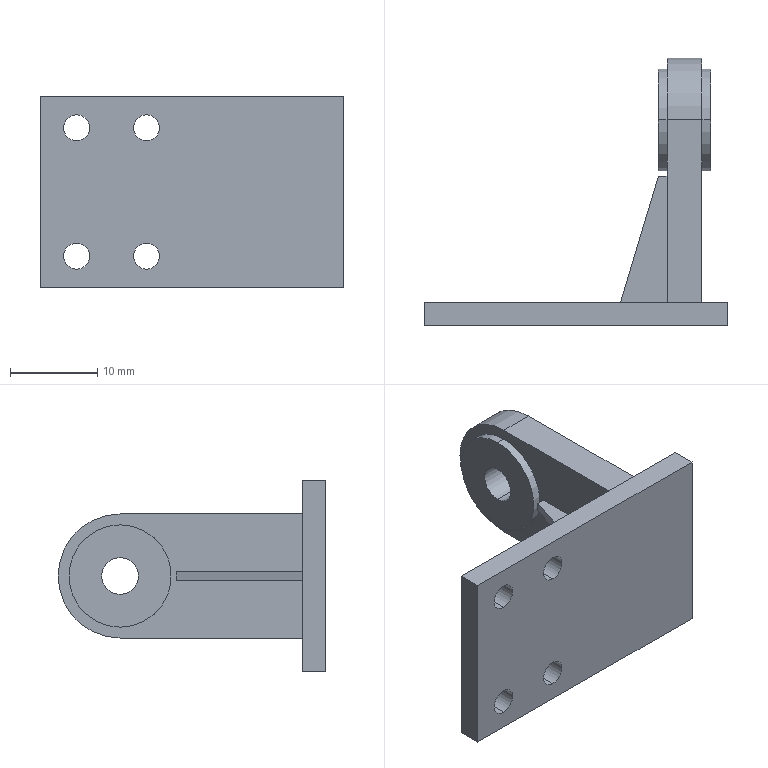Part | SolidWorks | features SavedExtBody 1 | 1 solid | 31 faces | box 34.775 x 30.759 x 22 mm | volume 3678 mm3 | plane 16 | cylinder 15 | commonest cylinder face diameters 3 x8 11.749 x4 4.217 x2 14.248 x1
STEP:
#1=CARTESIAN_POINT('',(69.335,-225.404,73.872));
#2=VERTEX_POINT('',#1);
#3=CARTESIAN_POINT('',(69.335,-225.404,70.872));
#4=VERTEX_POINT('',#3);
#5=CARTESIAN_POINT('',(69.335,-225.404,72.372));
#6=DIRECTION('',(0.,-1.,0.));
#7=DIRECTION('',(0.,0.,-1.));
#8=AXIS2_PLACEMENT_3D('',#5,#6,#7);
#9=CIRCLE('',#8,1.5);
#10=EDGE_CURVE('',#2,#4,#9,.T.);
#11=ORIENTED_EDGE('',*,*,#10,.F.);
#12=CARTESIAN_POINT('',(69.335,-228.101,73.872));
#13=VERTEX_POINT('',#12);
#14=CARTESIAN_POINT('',(69.335,-217.763,73.872));
#15=DIRECTION('',(0.,-1.,0.));
#16=VECTOR('',#15,1000.);
#17=LINE('',#14,#16);
#18=EDGE_CURVE('',#2,#13,#17,.T.);
#19=ORIENTED_EDGE('',*,*,#18,.T.);
#20=CARTESIAN_POINT('',(69.335,-228.101,70.872));
#21=VERTEX_POINT('',#20);
#22=CARTESIAN_POINT('',(69.335,-228.101,72.372));
#23=DIRECTION('',(0.,1.,0.));
#24=DIRECTION('',(0.,0.,1.));
#25=AXIS2_PLACEMENT_3D('',#22,#23,#24);
#26=CIRCLE('',#25,1.5);
#27=EDGE_CURVE('',#21,#13,#26,.T.);
#28=ORIENTED_EDGE('',*,*,#27,.F.);
#29=CARTESIAN_POINT('',(69.335,-217.763,70.872));
#30=DIRECTION('',(0.,-1.,0.));
#31=VECTOR('',#30,1000.);
#32=LINE('',#29,#31);
#33=EDGE_CURVE('',#4,#21,#32,.T.);
#34=ORIENTED_EDGE('',*,*,#33,.F.);
#35=EDGE_LOOP('',(#11,#19,#28,#34));
#36=FACE_OUTER_BOUND('',#35,.T.);
#37=CARTESIAN_POINT('',(69.335,-217.763,72.372));
#38=DIRECTION('',(0.,-1.,0.));
#39=DIRECTION('',(0.,0.,-1.));
#40=AXIS2_PLACEMENT_3D('',#37,#38,#39);
#41=CYLINDRICAL_SURFACE('',#40,1.5);
#42=ADVANCED_FACE('',(#36),#41,.F.);
#43=CARTESIAN_POINT('',(77.361,-225.404,73.872));
#44=VERTEX_POINT('',#43);
#45=CARTESIAN_POINT('',(77.361,-225.404,70.872));
#46=VERTEX_POINT('',#45);
#47=CARTESIAN_POINT('',(77.361,-225.404,72.372));
#48=DIRECTION('',(0.,-1.,0.));
#49=DIRECTION('',(0.,0.,-1.));
#50=AXIS2_PLACEMENT_3D('',#47,#48,#49);
#51=CIRCLE('',#50,1.5);
#52=EDGE_CURVE('',#44,#46,#51,.T.);
#53=ORIENTED_EDGE('',*,*,#52,.F.);
#54=CARTESIAN_POINT('',(77.361,-228.101,73.872));
#55=VERTEX_POINT('',#54);
#56=CARTESIAN_POINT('',(77.361,-217.763,73.872));
#57=DIRECTION('',(0.,-1.,0.));
#58=VECTOR('',#57,1000.);
#59=LINE('',#56,#58);
#60=EDGE_CURVE('',#44,#55,#59,.T.);
#61=ORIENTED_EDGE('',*,*,#60,.T.);
#62=CARTESIAN_POINT('',(77.361,-228.101,70.872));
#63=VERTEX_POINT('',#62);
#64=CARTESIAN_POINT('',(77.361,-228.101,72.372));
#65=DIRECTION('',(0.,1.,0.));
#66=DIRECTION('',(0.,0.,1.));
#67=AXIS2_PLACEMENT_3D('',#64,#65,#66);
#68=CIRCLE('',#67,1.5);
#69=EDGE_CURVE('',#63,#55,#68,.T.);
#70=ORIENTED_EDGE('',*,*,#69,.F.);
#71=CARTESIAN_POINT('',(77.361,-217.763,70.872));
#72=DIRECTION('',(0.,-1.,0.));
#73=VECTOR('',#72,1000.);
#74=LINE('',#71,#73);
#75=EDGE_CURVE('',#46,#63,#74,.T.);
#76=ORIENTED_EDGE('',*,*,#75,.F.);
#77=EDGE_LOOP('',(#53,#61,#70,#76));
#78=FACE_OUTER_BOUND('',#77,.T.);
#79=CARTESIAN_POINT('',(77.361,-217.763,72.372));
#80=DIRECTION('',(0.,-1.,0.));
#81=DIRECTION('',(0.,0.,-1.));
#82=AXIS2_PLACEMENT_3D('',#79,#80,#81);
#83=CYLINDRICAL_SURFACE('',#82,1.5);
#84=ADVANCED_FACE('',(#78),#83,.F.);
#85=CARTESIAN_POINT('',(77.361,-225.404,59.128));
#86=VERTEX_POINT('',#85);
#87=CARTESIAN_POINT('',(77.361,-225.404,56.128));
#88=VERTEX_POINT('',#87);
#89=CARTESIAN_POINT('',(77.361,-225.404,57.628));
#90=DIRECTION('',(0.,-1.,0.));
#91=DIRECTION('',(0.,0.,-1.));
#92=AXIS2_PLACEMENT_3D('',#89,#90,#91);
#93=CIRCLE('',#92,1.5);
#94=EDGE_CURVE('',#86,#88,#93,.T.);
#95=ORIENTED_EDGE('',*,*,#94,.F.);
#96=CARTESIAN_POINT('',(77.361,-228.101,59.128));
#97=VERTEX_POINT('',#96);
#98=CARTESIAN_POINT('',(77.361,-217.763,59.128));
#99=DIRECTION('',(0.,-1.,0.));
#100=VECTOR('',#99,1000.);
#101=LINE('',#98,#100);
#102=EDGE_CURVE('',#86,#97,#101,.T.);
#103=ORIENTED_EDGE('',*,*,#102,.T.);
#104=CARTESIAN_POINT('',(77.361,-228.101,56.128));
#105=VERTEX_POINT('',#104);
#106=CARTESIAN_POINT('',(77.361,-228.101,57.628));
#107=DIRECTION('',(0.,1.,0.));
#108=DIRECTION('',(0.,0.,1.));
#109=AXIS2_PLACEMENT_3D('',#106,#107,#108);
#110=CIRCLE('',#109,1.5);
#111=EDGE_CURVE('',#105,#97,#110,.T.);
#112=ORIENTED_EDGE('',*,*,#111,.F.);
#113=CARTESIAN_POINT('',(77.361,-217.763,56.128));
#114=DIRECTION('',(0.,-1.,0.));
#115=VECTOR('',#114,1000.);
#116=LINE('',#113,#115);
#117=EDGE_CURVE('',#88,#105,#116,.T.);
#118=ORIENTED_EDGE('',*,*,#117,.F.);
#119=EDGE_LOOP('',(#95,#103,#112,#118));
#120=FACE_OUTER_BOUND('',#119,.T.);
#121=CARTESIAN_POINT('',(77.361,-217.763,57.628));
#122=DIRECTION('',(0.,-1.,0.));
#123=DIRECTION('',(0.,0.,-1.));
#124=AXIS2_PLACEMENT_3D('',#121,#122,#123);
#125=CYLINDRICAL_SURFACE('',#124,1.5);
#126=ADVANCED_FACE('',(#120),#125,.F.);
#127=CARTESIAN_POINT('',(69.335,-225.404,59.128));
#128=VERTEX_POINT('',#127);
#129=CARTESIAN_POINT('',(69.335,-225.404,56.128));
#130=VERTEX_POINT('',#129);
#131=CARTESIAN_POINT('',(69.335,-225.404,57.628));
#132=DIRECTION('',(0.,-1.,0.));
#133=DIRECTION('',(0.,0.,-1.));
#134=AXIS2_PLACEMENT_3D('',#131,#132,#133);
#135=CIRCLE('',#134,1.5);
#136=EDGE_CURVE('',#128,#130,#135,.T.);
#137=ORIENTED_EDGE('',*,*,#136,.F.);
#138=CARTESIAN_POINT('',(69.335,-228.101,59.128));
#139=VERTEX_POINT('',#138);
#140=CARTESIAN_POINT('',(69.335,-217.763,59.128));
#141=DIRECTION('',(0.,-1.,0.));
#142=VECTOR('',#141,1000.);
#143=LINE('',#140,#142);
#144=EDGE_CURVE('',#128,#139,#143,.T.);
#145=ORIENTED_EDGE('',*,*,#144,.T.);
#146=CARTESIAN_POINT('',(69.335,-228.101,56.128));
#147=VERTEX_POINT('',#146);
#148=CARTESIAN_POINT('',(69.335,-228.101,57.628));
#149=DIRECTION('',(0.,1.,0.));
#150=DIRECTION('',(0.,0.,1.));
#151=AXIS2_PLACEMENT_3D('',#148,#149,#150);
#152=CIRCLE('',#151,1.5);
#153=EDGE_CURVE('',#147,#139,#152,.T.);
#154=ORIENTED_EDGE('',*,*,#153,.F.);
#155=CARTESIAN_POINT('',(69.335,-217.763,56.128));
#156=DIRECTION('',(0.,-1.,0.));
#157=VECTOR('',#156,1000.);
#158=LINE('',#155,#157);
#159=EDGE_CURVE('',#130,#147,#158,.T.);
#160=ORIENTED_EDGE('',*,*,#159,.F.);
#161=EDGE_LOOP('',(#137,#145,#154,#160));
#162=FACE_OUTER_BOUND('',#161,.T.);
#163=CARTESIAN_POINT('',(69.335,-217.763,57.628));
#164=DIRECTION('',(0.,-1.,0.));
#165=DIRECTION('',(0.,0.,-1.));
#166=AXIS2_PLACEMENT_3D('',#163,#164,#165);
#167=CYLINDRICAL_SURFACE('',#166,1.5);
#168=ADVANCED_FACE('',(#162),#167,.F.);
#169=CARTESIAN_POINT('',(92.041,-204.466,67.108));
#170=VERTEX_POINT('',#169);
#171=CARTESIAN_POINT('',(92.041,-204.466,62.892));
#172=VERTEX_POINT('',#171);
#173=CARTESIAN_POINT('',(92.041,-204.466,65.));
#174=DIRECTION('',(1.,0.,0.));
#175=DIRECTION('',(0.,0.,-1.));
#176=AXIS2_PLACEMENT_3D('',#173,#174,#175);
#177=CIRCLE('',#176,2.108);
#178=EDGE_CURVE('',#170,#172,#177,.T.);
#179=ORIENTED_EDGE('',*,*,#178,.F.);
#180=CARTESIAN_POINT('',(98.041,-204.466,67.108));
#181=VERTEX_POINT('',#180);
#182=CARTESIAN_POINT('',(100.386,-204.466,67.108));
#183=DIRECTION('',(1.,0.,0.));
#184=VECTOR('',#183,1000.);
#185=LINE('',#182,#184);
#186=EDGE_CURVE('',#170,#181,#185,.T.);
#187=ORIENTED_EDGE('',*,*,#186,.T.);
#188=CARTESIAN_POINT('',(98.041,-204.466,62.892));
#189=VERTEX_POINT('',#188);
#190=CARTESIAN_POINT('',(98.041,-204.466,65.));
#191=DIRECTION('',(1.,0.,0.));
#192=DIRECTION('',(0.,0.,-1.));
#193=AXIS2_PLACEMENT_3D('',#190,#191,#192);
#194=CIRCLE('',#193,2.108);
#195=EDGE_CURVE('',#181,#189,#194,.T.);
#196=ORIENTED_EDGE('',*,*,#195,.T.);
#197=CARTESIAN_POINT('',(100.386,-204.466,62.892));
#198=DIRECTION('',(1.,0.,0.));
#199=VECTOR('',#198,1000.);
#200=LINE('',#197,#199);
#201=EDGE_CURVE('',#172,#189,#200,.T.);
#202=ORIENTED_EDGE('',*,*,#201,.F.);
#203=EDGE_LOOP('',(#179,#187,#196,#202));
#204=FACE_OUTER_BOUND('',#203,.T.);
#205=CARTESIAN_POINT('',(100.386,-204.466,65.));
#206=DIRECTION('',(1.,0.,0.));
#207=DIRECTION('',(0.,0.,-1.));
#208=AXIS2_PLACEMENT_3D('',#205,#206,#207);
#209=CYLINDRICAL_SURFACE('',#208,2.108);
#210=ADVANCED_FACE('',(#204),#209,.F.);
#211=CARTESIAN_POINT('',(98.041,-204.466,59.125));
#212=VERTEX_POINT('',#211);
#213=CARTESIAN_POINT('',(98.041,-204.466,70.875));
#214=VERTEX_POINT('',#213);
#215=CARTESIAN_POINT('',(98.041,-204.466,65.));
#216=DIRECTION('',(1.,0.,0.));
#217=DIRECTION('',(0.,0.,-1.));
#218=AXIS2_PLACEMENT_3D('',#215,#216,#217);
#219=CIRCLE('',#218,5.875);
#220=EDGE_CURVE('',#212,#214,#219,.T.);
#221=ORIENTED_EDGE('',*,*,#220,.F.);
#222=CARTESIAN_POINT('',(97.041,-204.466,59.125));
#223=VERTEX_POINT('',#222);
#224=CARTESIAN_POINT('',(98.041,-204.466,59.125));
#225=DIRECTION('',(-1.,0.,0.));
#226=VECTOR('',#225,1000.);
#227=LINE('',#224,#226);
#228=EDGE_CURVE('',#212,#223,#227,.T.);
#229=ORIENTED_EDGE('',*,*,#228,.T.);
#230=CARTESIAN_POINT('',(97.041,-204.466,70.875));
#231=VERTEX_POINT('',#230);
#232=CARTESIAN_POINT('',(97.041,-204.466,65.));
#233=DIRECTION('',(-1.,0.,0.));
#234=DIRECTION('',(0.,0.,-1.));
#235=AXIS2_PLACEMENT_3D('',#232,#233,#234);
#236=CIRCLE('',#235,5.875);
#237=EDGE_CURVE('',#231,#223,#236,.T.);
#238=ORIENTED_EDGE('',*,*,#237,.F.);
#239=CARTESIAN_POINT('',(98.041,-204.466,70.875));
#240=DIRECTION('',(-1.,0.,0.));
#241=VECTOR('',#240,1000.);
#242=LINE('',#239,#241);
#243=EDGE_CURVE('',#214,#231,#242,.T.);
#244=ORIENTED_EDGE('',*,*,#243,.F.);
#245=EDGE_LOOP('',(#221,#229,#238,#244));
#246=FACE_OUTER_BOUND('',#245,.T.);
#247=CARTESIAN_POINT('',(98.041,-204.466,65.));
#248=DIRECTION('',(-1.,0.,0.));
#249=DIRECTION('',(0.,0.,1.));
#250=AXIS2_PLACEMENT_3D('',#247,#248,#249);
#251=CYLINDRICAL_SURFACE('',#250,5.875);
#252=ADVANCED_FACE('',(#246),#251,.T.);
#253=CARTESIAN_POINT('',(93.041,-204.466,70.875));
#254=VERTEX_POINT('',#253);
#255=CARTESIAN_POINT('',(93.041,-204.466,59.125));
#256=VERTEX_POINT('',#255);
#257=CARTESIAN_POINT('',(93.041,-204.466,65.));
#258=DIRECTION('',(-1.,0.,0.));
#259=DIRECTION('',(0.,0.,-1.));
#260=AXIS2_PLACEMENT_3D('',#257,#258,#259);
#261=CIRCLE('',#260,5.875);
#262=EDGE_CURVE('',#254,#256,#261,.T.);
#263=ORIENTED_EDGE('',*,*,#262,.T.);
#264=CARTESIAN_POINT('',(92.041,-204.466,59.125));
#265=VERTEX_POINT('',#264);
#266=CARTESIAN_POINT('',(98.041,-204.466,59.125));
#267=DIRECTION('',(-1.,0.,0.));
#268=VECTOR('',#267,1000.);
#269=LINE('',#266,#268);
#270=EDGE_CURVE('',#256,#265,#269,.T.);
#271=ORIENTED_EDGE('',*,*,#270,.T.);
#272=CARTESIAN_POINT('',(92.041,-204.466,70.875));
#273=VERTEX_POINT('',#272);
#274=CARTESIAN_POINT('',(92.041,-204.466,65.));
#275=DIRECTION('',(1.,0.,0.));
#276=DIRECTION('',(0.,0.,-1.));
#277=AXIS2_PLACEMENT_3D('',#274,#275,#276);
#278=CIRCLE('',#277,5.875);
#279=EDGE_CURVE('',#265,#273,#278,.T.);
#280=ORIENTED_EDGE('',*,*,#279,.T.);
#281=CARTESIAN_POINT('',(98.041,-204.466,70.875));
#282=DIRECTION('',(-1.,0.,0.));
#283=VECTOR('',#282,1000.);
#284=LINE('',#281,#283);
#285=EDGE_CURVE('',#254,#273,#284,.T.);
#286=ORIENTED_EDGE('',*,*,#285,.F.);
#287=EDGE_LOOP('',(#263,#271,#280,#286));
#288=FACE_OUTER_BOUND('',#287,.T.);
#289=CARTESIAN_POINT('',(98.041,-204.466,65.));
#290=DIRECTION('',(-1.,0.,0.));
#291=DIRECTION('',(0.,0.,1.));
#292=AXIS2_PLACEMENT_3D('',#289,#290,#291);
#293=CYLINDRICAL_SURFACE('',#292,5.875);
#294=ADVANCED_FACE('',(#288),#293,.T.);
#295=CARTESIAN_POINT('',(65.198,-225.404,54.));
#296=VERTEX_POINT('',#295);
#297=CARTESIAN_POINT('',(65.198,-228.101,54.));
#298=VERTEX_POINT('',#297);
#299=CARTESIAN_POINT('',(65.198,-228.101,54.));
#300=DIRECTION('',(0.,-1.,0.));
#301=VECTOR('',#300,1000.);
#302=LINE('',#299,#301);
#303=EDGE_CURVE('',#296,#298,#302,.T.);
#304=ORIENTED_EDGE('',*,*,#303,.T.);
#305=CARTESIAN_POINT('',(65.198,-228.101,76.));
#306=VERTEX_POINT('',#305);
#307=CARTESIAN_POINT('',(65.198,-228.101,76.));
#308=DIRECTION('',(0.,0.,-1.));
#309=VECTOR('',#308,1000.);
#310=LINE('',#307,#309);
#311=EDGE_CURVE('',#306,#298,#310,.T.);
#312=ORIENTED_EDGE('',*,*,#311,.F.);
#313=CARTESIAN_POINT('',(65.198,-225.404,76.));
#314=VERTEX_POINT('',#313);
#315=CARTESIAN_POINT('',(65.198,-228.101,76.));
#316=DIRECTION('',(0.,-1.,0.));
#317=VECTOR('',#316,1000.);
#318=LINE('',#315,#317);
#319=EDGE_CURVE('',#314,#306,#318,.T.);
#320=ORIENTED_EDGE('',*,*,#319,.F.);
#321=CARTESIAN_POINT('',(65.198,-225.404,76.));
#322=DIRECTION('',(0.,0.,-1.));
#323=VECTOR('',#322,1000.);
#324=LINE('',#321,#323);
#325=EDGE_CURVE('',#314,#296,#324,.T.);
#326=ORIENTED_EDGE('',*,*,#325,.T.);
#327=EDGE_LOOP('',(#304,#312,#320,#326));
#328=FACE_OUTER_BOUND('',#327,.T.);
#329=CARTESIAN_POINT('',(65.198,-228.101,76.));
#330=DIRECTION('',(1.,0.,0.));
#331=DIRECTION('',(0.,0.,-1.));
#332=AXIS2_PLACEMENT_3D('',#329,#330,#331);
#333=PLANE('',#332);
#334=ADVANCED_FACE('',(#328),#333,.F.);
#335=ORIENTED_EDGE('',*,*,#27,.T.);
#336=CARTESIAN_POINT('',(69.335,-228.101,72.372));
#337=DIRECTION('',(0.,1.,0.));
#338=DIRECTION('',(0.,0.,1.));
#339=AXIS2_PLACEMENT_3D('',#336,#337,#338);
#340=CIRCLE('',#339,1.5);
#341=EDGE_CURVE('',#13,#21,#340,.T.);
#342=ORIENTED_EDGE('',*,*,#341,.T.);
#343=EDGE_LOOP('',(#335,#342));
#344=FACE_BOUND('',#343,.T.);
#345=ORIENTED_EDGE('',*,*,#69,.T.);
#346=CARTESIAN_POINT('',(77.361,-228.101,72.372));
#347=DIRECTION('',(0.,1.,0.));
#348=DIRECTION('',(0.,0.,1.));
#349=AXIS2_PLACEMENT_3D('',#346,#347,#348);
#350=CIRCLE('',#349,1.5);
#351=EDGE_CURVE('',#55,#63,#350,.T.);
#352=ORIENTED_EDGE('',*,*,#351,.T.);
#353=EDGE_LOOP('',(#345,#352));
#354=FACE_BOUND('',#353,.T.);
#355=ORIENTED_EDGE('',*,*,#111,.T.);
#356=CARTESIAN_POINT('',(77.361,-228.101,57.628));
#357=DIRECTION('',(0.,1.,0.));
#358=DIRECTION('',(0.,0.,1.));
#359=AXIS2_PLACEMENT_3D('',#356,#357,#358);
#360=CIRCLE('',#359,1.5);
#361=EDGE_CURVE('',#97,#105,#360,.T.);
#362=ORIENTED_EDGE('',*,*,#361,.T.);
#363=EDGE_LOOP('',(#355,#362));
#364=FACE_BOUND('',#363,.T.);
#365=ORIENTED_EDGE('',*,*,#153,.T.);
#366=CARTESIAN_POINT('',(69.335,-228.101,57.628));
#367=DIRECTION('',(0.,1.,0.));
#368=DIRECTION('',(0.,0.,1.));
#369=AXIS2_PLACEMENT_3D('',#366,#367,#368);
#370=CIRCLE('',#369,1.5);
#371=EDGE_CURVE('',#139,#147,#370,.T.);
#372=ORIENTED_EDGE('',*,*,#371,.T.);
#373=EDGE_LOOP('',(#365,#372));
#374=FACE_BOUND('',#373,.T.);
#375=CARTESIAN_POINT('',(99.974,-228.101,54.));
#376=VERTEX_POINT('',#375);
#377=CARTESIAN_POINT('',(65.198,-228.101,54.));
#378=DIRECTION('',(1.,0.,0.));
#379=VECTOR('',#378,1000.);
#380=LINE('',#377,#379);
#381=EDGE_CURVE('',#298,#376,#380,.T.);
#382=ORIENTED_EDGE('',*,*,#381,.T.);
#383=CARTESIAN_POINT('',(99.974,-228.101,76.));
#384=VERTEX_POINT('',#383);
#385=CARTESIAN_POINT('',(99.974,-228.101,76.));
#386=DIRECTION('',(0.,0.,-1.));
#387=VECTOR('',#386,1000.);
#388=LINE('',#385,#387);
#389=EDGE_CURVE('',#384,#376,#388,.T.);
#390=ORIENTED_EDGE('',*,*,#389,.F.);
#391=CARTESIAN_POINT('',(65.198,-228.101,76.));
#392=DIRECTION('',(1.,0.,0.));
#393=VECTOR('',#392,1000.);
#394=LINE('',#391,#393);
#395=EDGE_CURVE('',#306,#384,#394,.T.);
#396=ORIENTED_EDGE('',*,*,#395,.F.);
#397=ORIENTED_EDGE('',*,*,#311,.T.);
#398=EDGE_LOOP('',(#382,#390,#396,#397));
#399=FACE_OUTER_BOUND('',#398,.T.);
#400=CARTESIAN_POINT('',(65.198,-228.101,76.));
#401=DIRECTION('',(0.,1.,0.));
#402=DIRECTION('',(0.,0.,1.));
#403=AXIS2_PLACEMENT_3D('',#400,#401,#402);
#404=PLANE('',#403);
#405=ADVANCED_FACE('',(#344,#354,#364,#374,#399),#404,.F.);
#406=CARTESIAN_POINT('',(99.974,-225.404,54.));
#407=VERTEX_POINT('',#406);
#408=CARTESIAN_POINT('',(99.974,-228.101,54.));
#409=DIRECTION('',(0.,1.,0.));
#410=VECTOR('',#409,1000.);
#411=LINE('',#408,#410);
#412=EDGE_CURVE('',#376,#407,#411,.T.);
#413=ORIENTED_EDGE('',*,*,#412,.T.);
#414=CARTESIAN_POINT('',(99.974,-225.404,76.));
#415=VERTEX_POINT('',#414);
#416=CARTESIAN_POINT('',(99.974,-225.404,76.));
#417=DIRECTION('',(0.,0.,-1.));
#418=VECTOR('',#417,1000.);
#419=LINE('',#416,#418);
#420=EDGE_CURVE('',#415,#407,#419,.T.);
#421=ORIENTED_EDGE('',*,*,#420,.F.);
#422=CARTESIAN_POINT('',(99.974,-228.101,76.));
#423=DIRECTION('',(0.,1.,0.));
#424=VECTOR('',#423,1000.);
#425=LINE('',#422,#424);
#426=EDGE_CURVE('',#384,#415,#425,.T.);
#427=ORIENTED_EDGE('',*,*,#426,.F.);
#428=ORIENTED_EDGE('',*,*,#389,.T.);
#429=EDGE_LOOP('',(#413,#421,#427,#428));
#430=FACE_OUTER_BOUND('',#429,.T.);
#431=CARTESIAN_POINT('',(99.974,-228.101,76.));
#432=DIRECTION('',(-1.,0.,0.));
#433=DIRECTION('',(0.,0.,1.));
#434=AXIS2_PLACEMENT_3D('',#431,#432,#433);
#435=PLANE('',#434);
#436=ADVANCED_FACE('',(#430),#435,.F.);
#437=CARTESIAN_POINT('',(69.335,-225.404,72.372));
#438=DIRECTION('',(0.,-1.,0.));
#439=DIRECTION('',(0.,0.,-1.));
#440=AXIS2_PLACEMENT_3D('',#437,#438,#439);
#441=CIRCLE('',#440,1.5);
#442=EDGE_CURVE('',#4,#2,#441,.T.);
#443=ORIENTED_EDGE('',*,*,#442,.T.);
#444=ORIENTED_EDGE('',*,*,#10,.T.);
#445=EDGE_LOOP('',(#443,#444));
#446=FACE_BOUND('',#445,.T.);
#447=CARTESIAN_POINT('',(77.361,-225.404,72.372));
#448=DIRECTION('',(0.,-1.,0.));
#449=DIRECTION('',(0.,0.,-1.));
#450=AXIS2_PLACEMENT_3D('',#447,#448,#449);
#451=CIRCLE('',#450,1.5);
#452=EDGE_CURVE('',#46,#44,#451,.T.);
#453=ORIENTED_EDGE('',*,*,#452,.T.);
#454=ORIENTED_EDGE('',*,*,#52,.T.);
#455=EDGE_LOOP('',(#453,#454));
#456=FACE_BOUND('',#455,.T.);
#457=CARTESIAN_POINT('',(77.361,-225.404,57.628));
#458=DIRECTION('',(0.,-1.,0.));
#459=DIRECTION('',(0.,0.,-1.));
#460=AXIS2_PLACEMENT_3D('',#457,#458,#459);
#461=CIRCLE('',#460,1.5);
#462=EDGE_CURVE('',#88,#86,#461,.T.);
#463=ORIENTED_EDGE('',*,*,#462,.T.);
#464=ORIENTED_EDGE('',*,*,#94,.T.);
#465=EDGE_LOOP('',(#463,#464));
#466=FACE_BOUND('',#465,.T.);
#467=CARTESIAN_POINT('',(69.335,-225.404,57.628));
#468=DIRECTION('',(0.,-1.,0.));
#469=DIRECTION('',(0.,0.,-1.));
#470=AXIS2_PLACEMENT_3D('',#467,#468,#469);
#471=CIRCLE('',#470,1.5);
#472=EDGE_CURVE('',#130,#128,#471,.T.);
#473=ORIENTED_EDGE('',*,*,#472,.T.);
#474=ORIENTED_EDGE('',*,*,#136,.T.);
#475=EDGE_LOOP('',(#473,#474));
#476=FACE_BOUND('',#475,.T.);
#477=CARTESIAN_POINT('',(93.041,-225.404,72.124));
#478=VERTEX_POINT('',#477);
#479=CARTESIAN_POINT('',(93.041,-225.404,65.5));
#480=VERTEX_POINT('',#479);
#481=CARTESIAN_POINT('',(93.041,-225.404,72.124));
#482=DIRECTION('',(0.,0.,-1.));
#483=VECTOR('',#482,1000.);
#484=LINE('',#481,#483);
#485=EDGE_CURVE('',#478,#480,#484,.T.);
#486=ORIENTED_EDGE('',*,*,#485,.T.);
#487=CARTESIAN_POINT('',(87.693,-225.404,65.5));
#488=VERTEX_POINT('',#487);
#489=CARTESIAN_POINT('',(87.693,-225.404,65.5));
#490=DIRECTION('',(1.,0.,0.));
#491=VECTOR('',#490,1000.);
#492=LINE('',#489,#491);
#493=EDGE_CURVE('',#488,#480,#492,.T.);
#494=ORIENTED_EDGE('',*,*,#493,.F.);
#495=CARTESIAN_POINT('',(87.693,-225.404,64.5));
#496=VERTEX_POINT('',#495);
#497=CARTESIAN_POINT('',(87.693,-225.404,65.5));
#498=DIRECTION('',(0.,0.,-1.));
#499=VECTOR('',#498,1000.);
#500=LINE('',#497,#499);
#501=EDGE_CURVE('',#488,#496,#500,.T.);
#502=ORIENTED_EDGE('',*,*,#501,.T.);
#503=CARTESIAN_POINT('',(93.041,-225.404,64.5));
#504=VERTEX_POINT('',#503);
#505=CARTESIAN_POINT('',(87.693,-225.404,64.5));
#506=DIRECTION('',(1.,0.,0.));
#507=VECTOR('',#506,1000.);
#508=LINE('',#505,#507);
#509=EDGE_CURVE('',#496,#504,#508,.T.);
#510=ORIENTED_EDGE('',*,*,#509,.T.);
#511=CARTESIAN_POINT('',(93.041,-225.404,57.876));
#512=VERTEX_POINT('',#511);
#513=CARTESIAN_POINT('',(93.041,-225.404,72.124));
#514=DIRECTION('',(0.,0.,-1.));
#515=VECTOR('',#514,1000.);
#516=LINE('',#513,#515);
#517=EDGE_CURVE('',#504,#512,#516,.T.);
#518=ORIENTED_EDGE('',*,*,#517,.T.);
#519=CARTESIAN_POINT('',(97.041,-225.404,57.876));
#520=VERTEX_POINT('',#519);
#521=CARTESIAN_POINT('',(97.041,-225.404,57.876));
#522=DIRECTION('',(-1.,0.,0.));
#523=VECTOR('',#522,1000.);
#524=LINE('',#521,#523);
#525=EDGE_CURVE('',#520,#512,#524,.T.);
#526=ORIENTED_EDGE('',*,*,#525,.F.);
#527=CARTESIAN_POINT('',(97.041,-225.404,72.124));
#528=VERTEX_POINT('',#527);
#529=CARTESIAN_POINT('',(97.041,-225.404,72.124));
#530=DIRECTION('',(0.,0.,-1.));
#531=VECTOR('',#530,1000.);
#532=LINE('',#529,#531);
#533=EDGE_CURVE('',#528,#520,#532,.T.);
#534=ORIENTED_EDGE('',*,*,#533,.F.);
#535=CARTESIAN_POINT('',(97.041,-225.404,72.124));
#536=DIRECTION('',(-1.,0.,0.));
#537=VECTOR('',#536,1000.);
#538=LINE('',#535,#537);
#539=EDGE_CURVE('',#528,#478,#538,.T.);
#540=ORIENTED_EDGE('',*,*,#539,.T.);
#541=EDGE_LOOP('',(#486,#494,#502,#510,#518,#526,#534,#540));
#542=FACE_BOUND('',#541,.T.);
#543=CARTESIAN_POINT('',(65.198,-225.404,54.));
#544=DIRECTION('',(-1.,0.,0.));
#545=VECTOR('',#544,1000.);
#546=LINE('',#543,#545);
#547=EDGE_CURVE('',#407,#296,#546,.T.);
#548=ORIENTED_EDGE('',*,*,#547,.T.);
#549=ORIENTED_EDGE('',*,*,#325,.F.);
#550=CARTESIAN_POINT('',(65.198,-225.404,76.));
#551=DIRECTION('',(-1.,0.,0.));
#552=VECTOR('',#551,1000.);
#553=LINE('',#550,#552);
#554=EDGE_CURVE('',#415,#314,#553,.T.);
#555=ORIENTED_EDGE('',*,*,#554,.F.);
#556=ORIENTED_EDGE('',*,*,#420,.T.);
#557=EDGE_LOOP('',(#548,#549,#555,#556));
#558=FACE_OUTER_BOUND('',#557,.T.);
#559=CARTESIAN_POINT('',(65.198,-225.404,76.));
#560=DIRECTION('',(0.,-1.,0.));
#561=DIRECTION('',(0.,0.,-1.));
#562=AXIS2_PLACEMENT_3D('',#559,#560,#561);
#563=PLANE('',#562);
#564=ADVANCED_FACE('',(#446,#456,#466,#476,#542,#558),#563,.F.);
#565=ORIENTED_EDGE('',*,*,#319,.T.);
#566=ORIENTED_EDGE('',*,*,#395,.T.);
#567=ORIENTED_EDGE('',*,*,#426,.T.);
#568=ORIENTED_EDGE('',*,*,#554,.T.);
#569=EDGE_LOOP('',(#565,#566,#567,#568));
#570=FACE_OUTER_BOUND('',#569,.T.);
#571=CARTESIAN_POINT('',(0.,0.,76.));
#572=DIRECTION('',(0.,0.,-1.));
#573=DIRECTION('',(-1.,0.,0.));
#574=AXIS2_PLACEMENT_3D('',#571,#572,#573);
#575=PLANE('',#574);
#576=ADVANCED_FACE('',(#570),#575,.F.);
#577=ORIENTED_EDGE('',*,*,#303,.F.);
#578=ORIENTED_EDGE('',*,*,#547,.F.);
#579=ORIENTED_EDGE('',*,*,#412,.F.);
#580=ORIENTED_EDGE('',*,*,#381,.F.);
#581=EDGE_LOOP('',(#577,#578,#579,#580));
#582=FACE_OUTER_BOUND('',#581,.T.);
#583=CARTESIAN_POINT('',(0.,0.,54.));
#584=DIRECTION('',(0.,0.,-1.));
#585=DIRECTION('',(-1.,0.,0.));
#586=AXIS2_PLACEMENT_3D('',#583,#584,#585);
#587=PLANE('',#586);
#588=ADVANCED_FACE('',(#582),#587,.T.);
#589=CARTESIAN_POINT('',(93.041,-204.466,57.876));
#590=VERTEX_POINT('',#589);
#591=CARTESIAN_POINT('',(93.041,-204.466,72.124));
#592=VERTEX_POINT('',#591);
#593=CARTESIAN_POINT('',(93.041,-204.466,65.));
#594=DIRECTION('',(1.,0.,0.));
#595=DIRECTION('',(0.,0.,-1.));
#596=AXIS2_PLACEMENT_3D('',#593,#594,#595);
#597=CIRCLE('',#596,7.124);
#598=EDGE_CURVE('',#590,#592,#597,.T.);
#599=ORIENTED_EDGE('',*,*,#598,.T.);
#600=CARTESIAN_POINT('',(97.041,-204.466,72.124));
#601=VERTEX_POINT('',#600);
#602=CARTESIAN_POINT('',(97.041,-204.466,72.124));
#603=DIRECTION('',(-1.,0.,0.));
#604=VECTOR('',#603,1000.);
#605=LINE('',#602,#604);
#606=EDGE_CURVE('',#601,#592,#605,.T.);
#607=ORIENTED_EDGE('',*,*,#606,.F.);
#608=CARTESIAN_POINT('',(97.041,-204.466,57.876));
#609=VERTEX_POINT('',#608);
#610=CARTESIAN_POINT('',(97.041,-204.466,65.));
#611=DIRECTION('',(1.,0.,0.));
#612=DIRECTION('',(0.,0.,-1.));
#613=AXIS2_PLACEMENT_3D('',#610,#611,#612);
#614=CIRCLE('',#613,7.124);
#615=EDGE_CURVE('',#609,#601,#614,.T.);
#616=ORIENTED_EDGE('',*,*,#615,.F.);
#617=CARTESIAN_POINT('',(97.041,-204.466,57.876));
#618=DIRECTION('',(-1.,0.,0.));
#619=VECTOR('',#618,1000.);
#620=LINE('',#617,#619);
#621=EDGE_CURVE('',#609,#590,#620,.T.);
#622=ORIENTED_EDGE('',*,*,#621,.T.);
#623=EDGE_LOOP('',(#599,#607,#616,#622));
#624=FACE_OUTER_BOUND('',#623,.T.);
#625=CARTESIAN_POINT('',(97.041,-204.466,65.));
#626=DIRECTION('',(-1.,0.,0.));
#627=DIRECTION('',(0.,0.,1.));
#628=AXIS2_PLACEMENT_3D('',#625,#626,#627);
#629=CYLINDRICAL_SURFACE('',#628,7.124);
#630=ADVANCED_FACE('',(#624),#629,.T.);
#631=CARTESIAN_POINT('',(93.041,-204.466,72.124));
#632=DIRECTION('',(0.,-1.,0.));
#633=VECTOR('',#632,1000.);
#634=LINE('',#631,#633);
#635=EDGE_CURVE('',#592,#478,#634,.T.);
#636=ORIENTED_EDGE('',*,*,#635,.T.);
#637=ORIENTED_EDGE('',*,*,#539,.F.);
#638=CARTESIAN_POINT('',(97.041,-204.466,72.124));
#639=DIRECTION('',(0.,-1.,0.));
#640=VECTOR('',#639,1000.);
#641=LINE('',#638,#640);
#642=EDGE_CURVE('',#601,#528,#641,.T.);
#643=ORIENTED_EDGE('',*,*,#642,.F.);
#644=ORIENTED_EDGE('',*,*,#606,.T.);
#645=EDGE_LOOP('',(#636,#637,#643,#644));
#646=FACE_OUTER_BOUND('',#645,.T.);
#647=CARTESIAN_POINT('',(97.041,-204.466,72.124));
#648=DIRECTION('',(0.,0.,-1.));
#649=DIRECTION('',(-1.,0.,0.));
#650=AXIS2_PLACEMENT_3D('',#647,#648,#649);
#651=PLANE('',#650);
#652=ADVANCED_FACE('',(#646),#651,.F.);
#653=CARTESIAN_POINT('',(93.041,-225.404,57.876));
#654=DIRECTION('',(0.,1.,0.));
#655=VECTOR('',#654,1000.);
#656=LINE('',#653,#655);
#657=EDGE_CURVE('',#512,#590,#656,.T.);
#658=ORIENTED_EDGE('',*,*,#657,.T.);
#659=ORIENTED_EDGE('',*,*,#621,.F.);
#660=CARTESIAN_POINT('',(97.041,-225.404,57.876));
#661=DIRECTION('',(0.,1.,0.));
#662=VECTOR('',#661,1000.);
#663=LINE('',#660,#662);
#664=EDGE_CURVE('',#520,#609,#663,.T.);
#665=ORIENTED_EDGE('',*,*,#664,.F.);
#666=ORIENTED_EDGE('',*,*,#525,.T.);
#667=EDGE_LOOP('',(#658,#659,#665,#666));
#668=FACE_OUTER_BOUND('',#667,.T.);
#669=CARTESIAN_POINT('',(97.041,-225.404,57.876));
#670=DIRECTION('',(0.,0.,1.));
#671=DIRECTION('',(1.,0.,0.));
#672=AXIS2_PLACEMENT_3D('',#669,#670,#671);
#673=PLANE('',#672);
#674=ADVANCED_FACE('',(#668),#673,.F.);
#675=ORIENTED_EDGE('',*,*,#237,.T.);
#676=CARTESIAN_POINT('',(97.041,-204.466,65.));
#677=DIRECTION('',(-1.,0.,0.));
#678=DIRECTION('',(0.,0.,-1.));
#679=AXIS2_PLACEMENT_3D('',#676,#677,#678);
#680=CIRCLE('',#679,5.875);
#681=EDGE_CURVE('',#223,#231,#680,.T.);
#682=ORIENTED_EDGE('',*,*,#681,.T.);
#683=EDGE_LOOP('',(#675,#682));
#684=FACE_BOUND('',#683,.T.);
#685=ORIENTED_EDGE('',*,*,#615,.T.);
#686=ORIENTED_EDGE('',*,*,#642,.T.);
#687=ORIENTED_EDGE('',*,*,#533,.T.);
#688=ORIENTED_EDGE('',*,*,#664,.T.);
#689=EDGE_LOOP('',(#685,#686,#687,#688));
#690=FACE_OUTER_BOUND('',#689,.T.);
#691=CARTESIAN_POINT('',(97.041,-204.466,65.));
#692=DIRECTION('',(1.,0.,0.));
#693=DIRECTION('',(0.,0.,-1.));
#694=AXIS2_PLACEMENT_3D('',#691,#692,#693);
#695=PLANE('',#694);
#696=ADVANCED_FACE('',(#684,#690),#695,.T.);
#697=ORIENTED_EDGE('',*,*,#262,.F.);
#698=CARTESIAN_POINT('',(93.041,-204.466,65.));
#699=DIRECTION('',(-1.,0.,0.));
#700=DIRECTION('',(0.,0.,-1.));
#701=AXIS2_PLACEMENT_3D('',#698,#699,#700);
#702=CIRCLE('',#701,5.875);
#703=EDGE_CURVE('',#256,#254,#702,.T.);
#704=ORIENTED_EDGE('',*,*,#703,.F.);
#705=EDGE_LOOP('',(#697,#704));
#706=FACE_BOUND('',#705,.T.);
#707=CARTESIAN_POINT('',(93.041,-210.916,65.5));
#708=VERTEX_POINT('',#707);
#709=CARTESIAN_POINT('',(93.041,-210.916,64.5));
#710=VERTEX_POINT('',#709);
#711=CARTESIAN_POINT('',(93.041,-210.916,65.5));
#712=DIRECTION('',(0.,0.,-1.));
#713=VECTOR('',#712,1000.);
#714=LINE('',#711,#713);
#715=EDGE_CURVE('',#708,#710,#714,.T.);
#716=ORIENTED_EDGE('',*,*,#715,.F.);
#717=CARTESIAN_POINT('',(93.041,-225.404,65.5));
#718=DIRECTION('',(0.,1.,0.));
#719=VECTOR('',#718,1000.);
#720=LINE('',#717,#719);
#721=EDGE_CURVE('',#480,#708,#720,.T.);
#722=ORIENTED_EDGE('',*,*,#721,.F.);
#723=ORIENTED_EDGE('',*,*,#485,.F.);
#724=ORIENTED_EDGE('',*,*,#635,.F.);
#725=ORIENTED_EDGE('',*,*,#598,.F.);
#726=ORIENTED_EDGE('',*,*,#657,.F.);
#727=ORIENTED_EDGE('',*,*,#517,.F.);
#728=CARTESIAN_POINT('',(93.041,-225.404,64.5));
#729=DIRECTION('',(0.,1.,0.));
#730=VECTOR('',#729,1000.);
#731=LINE('',#728,#730);
#732=EDGE_CURVE('',#504,#710,#731,.T.);
#733=ORIENTED_EDGE('',*,*,#732,.T.);
#734=EDGE_LOOP('',(#716,#722,#723,#724,#725,#726,#727,#733));
#735=FACE_OUTER_BOUND('',#734,.T.);
#736=CARTESIAN_POINT('',(93.041,-204.466,65.));
#737=DIRECTION('',(1.,0.,0.));
#738=DIRECTION('',(0.,0.,-1.));
#739=AXIS2_PLACEMENT_3D('',#736,#737,#738);
#740=PLANE('',#739);
#741=ADVANCED_FACE('',(#706,#735),#740,.F.);
#742=CARTESIAN_POINT('',(92.041,-204.466,65.));
#743=DIRECTION('',(1.,0.,0.));
#744=DIRECTION('',(0.,0.,-1.));
#745=AXIS2_PLACEMENT_3D('',#742,#743,#744);
#746=CIRCLE('',#745,2.108);
#747=EDGE_CURVE('',#172,#170,#746,.T.);
#748=ORIENTED_EDGE('',*,*,#747,.T.);
#749=ORIENTED_EDGE('',*,*,#178,.T.);
#750=EDGE_LOOP('',(#748,#749));
#751=FACE_BOUND('',#750,.T.);
#752=CARTESIAN_POINT('',(92.041,-204.466,65.));
#753=DIRECTION('',(1.,0.,0.));
#754=DIRECTION('',(0.,0.,-1.));
#755=AXIS2_PLACEMENT_3D('',#752,#753,#754);
#756=CIRCLE('',#755,5.875);
#757=EDGE_CURVE('',#273,#265,#756,.T.);
#758=ORIENTED_EDGE('',*,*,#757,.F.);
#759=ORIENTED_EDGE('',*,*,#279,.F.);
#760=EDGE_LOOP('',(#758,#759));
#761=FACE_OUTER_BOUND('',#760,.T.);
#762=CARTESIAN_POINT('',(92.041,-204.466,65.));
#763=DIRECTION('',(1.,0.,0.));
#764=DIRECTION('',(0.,0.,-1.));
#765=AXIS2_PLACEMENT_3D('',#762,#763,#764);
#766=PLANE('',#765);
#767=ADVANCED_FACE('',(#751,#761),#766,.F.);
#768=ORIENTED_EDGE('',*,*,#270,.F.);
#769=ORIENTED_EDGE('',*,*,#703,.T.);
#770=ORIENTED_EDGE('',*,*,#285,.T.);
#771=ORIENTED_EDGE('',*,*,#757,.T.);
#772=EDGE_LOOP('',(#768,#769,#770,#771));
#773=FACE_OUTER_BOUND('',#772,.T.);
#774=CARTESIAN_POINT('',(98.041,-204.466,65.));
#775=DIRECTION('',(-1.,0.,0.));
#776=DIRECTION('',(0.,0.,1.));
#777=AXIS2_PLACEMENT_3D('',#774,#775,#776);
#778=CYLINDRICAL_SURFACE('',#777,5.875);
#779=ADVANCED_FACE('',(#773),#778,.T.);
#780=ORIENTED_EDGE('',*,*,#228,.F.);
#781=CARTESIAN_POINT('',(98.041,-204.466,65.));
#782=DIRECTION('',(1.,0.,0.));
#783=DIRECTION('',(0.,0.,-1.));
#784=AXIS2_PLACEMENT_3D('',#781,#782,#783);
#785=CIRCLE('',#784,5.875);
#786=EDGE_CURVE('',#214,#212,#785,.T.);
#787=ORIENTED_EDGE('',*,*,#786,.F.);
#788=ORIENTED_EDGE('',*,*,#243,.T.);
#789=ORIENTED_EDGE('',*,*,#681,.F.);
#790=EDGE_LOOP('',(#780,#787,#788,#789));
#791=FACE_OUTER_BOUND('',#790,.T.);
#792=CARTESIAN_POINT('',(98.041,-204.466,65.));
#793=DIRECTION('',(-1.,0.,0.));
#794=DIRECTION('',(0.,0.,1.));
#795=AXIS2_PLACEMENT_3D('',#792,#793,#794);
#796=CYLINDRICAL_SURFACE('',#795,5.875);
#797=ADVANCED_FACE('',(#791),#796,.T.);
#798=CARTESIAN_POINT('',(98.041,-204.466,65.));
#799=DIRECTION('',(1.,0.,0.));
#800=DIRECTION('',(0.,0.,-1.));
#801=AXIS2_PLACEMENT_3D('',#798,#799,#800);
#802=CIRCLE('',#801,2.108);
#803=EDGE_CURVE('',#189,#181,#802,.T.);
#804=ORIENTED_EDGE('',*,*,#803,.F.);
#805=ORIENTED_EDGE('',*,*,#195,.F.);
#806=EDGE_LOOP('',(#804,#805));
#807=FACE_BOUND('',#806,.T.);
#808=ORIENTED_EDGE('',*,*,#786,.T.);
#809=ORIENTED_EDGE('',*,*,#220,.T.);
#810=EDGE_LOOP('',(#808,#809));
#811=FACE_OUTER_BOUND('',#810,.T.);
#812=CARTESIAN_POINT('',(98.041,-204.466,65.));
#813=DIRECTION('',(1.,0.,0.));
#814=DIRECTION('',(0.,0.,-1.));
#815=AXIS2_PLACEMENT_3D('',#812,#813,#814);
#816=PLANE('',#815);
#817=ADVANCED_FACE('',(#807,#811),#816,.T.);
#818=CARTESIAN_POINT('',(92.041,-210.916,64.5));
#819=VERTEX_POINT('',#818);
#820=CARTESIAN_POINT('',(93.041,-210.916,64.5));
#821=DIRECTION('',(-1.,0.,0.));
#822=VECTOR('',#821,1000.);
#823=LINE('',#820,#822);
#824=EDGE_CURVE('',#710,#819,#823,.T.);
#825=ORIENTED_EDGE('',*,*,#824,.T.);
#826=CARTESIAN_POINT('',(92.041,-210.916,65.5));
#827=VERTEX_POINT('',#826);
#828=CARTESIAN_POINT('',(92.041,-210.916,65.5));
#829=DIRECTION('',(0.,0.,-1.));
#830=VECTOR('',#829,1000.);
#831=LINE('',#828,#830);
#832=EDGE_CURVE('',#827,#819,#831,.T.);
#833=ORIENTED_EDGE('',*,*,#832,.F.);
#834=CARTESIAN_POINT('',(93.041,-210.916,65.5));
#835=DIRECTION('',(-1.,0.,0.));
#836=VECTOR('',#835,1000.);
#837=LINE('',#834,#836);
#838=EDGE_CURVE('',#708,#827,#837,.T.);
#839=ORIENTED_EDGE('',*,*,#838,.F.);
#840=ORIENTED_EDGE('',*,*,#715,.T.);
#841=EDGE_LOOP('',(#825,#833,#839,#840));
#842=FACE_OUTER_BOUND('',#841,.T.);
#843=CARTESIAN_POINT('',(93.041,-210.916,65.5));
#844=DIRECTION('',(0.,-1.,0.));
#845=DIRECTION('',(0.,0.,-1.));
#846=AXIS2_PLACEMENT_3D('',#843,#844,#845);
#847=PLANE('',#846);
#848=ADVANCED_FACE('',(#842),#847,.F.);
#849=CARTESIAN_POINT('',(92.041,-210.916,64.5));
#850=DIRECTION('',(-0.2874,-0.9578,0.));
#851=VECTOR('',#850,1000.);
#852=LINE('',#849,#851);
#853=EDGE_CURVE('',#819,#496,#852,.T.);
#854=ORIENTED_EDGE('',*,*,#853,.T.);
#855=ORIENTED_EDGE('',*,*,#501,.F.);
#856=CARTESIAN_POINT('',(92.041,-210.916,65.5));
#857=DIRECTION('',(-0.2874,-0.9578,0.));
#858=VECTOR('',#857,1000.);
#859=LINE('',#856,#858);
#860=EDGE_CURVE('',#827,#488,#859,.T.);
#861=ORIENTED_EDGE('',*,*,#860,.F.);
#862=ORIENTED_EDGE('',*,*,#832,.T.);
#863=EDGE_LOOP('',(#854,#855,#861,#862));
#864=FACE_OUTER_BOUND('',#863,.T.);
#865=CARTESIAN_POINT('',(92.041,-210.916,65.5));
#866=DIRECTION('',(0.9578,-0.2874,0.));
#867=DIRECTION('',(0.2874,0.9578,0.));
#868=AXIS2_PLACEMENT_3D('',#865,#866,#867);
#869=PLANE('',#868);
#870=ADVANCED_FACE('',(#864),#869,.F.);
#871=ORIENTED_EDGE('',*,*,#721,.T.);
#872=ORIENTED_EDGE('',*,*,#838,.T.);
#873=ORIENTED_EDGE('',*,*,#860,.T.);
#874=ORIENTED_EDGE('',*,*,#493,.T.);
#875=EDGE_LOOP('',(#871,#872,#873,#874));
#876=FACE_OUTER_BOUND('',#875,.T.);
#877=CARTESIAN_POINT('',(0.,0.,65.5));
#878=DIRECTION('',(0.,0.,1.));
#879=DIRECTION('',(1.,0.,0.));
#880=AXIS2_PLACEMENT_3D('',#877,#878,#879);
#881=PLANE('',#880);
#882=ADVANCED_FACE('',(#876),#881,.T.);
#883=ORIENTED_EDGE('',*,*,#732,.F.);
#884=ORIENTED_EDGE('',*,*,#509,.F.);
#885=ORIENTED_EDGE('',*,*,#853,.F.);
#886=ORIENTED_EDGE('',*,*,#824,.F.);
#887=EDGE_LOOP('',(#883,#884,#885,#886));
#888=FACE_OUTER_BOUND('',#887,.T.);
#889=CARTESIAN_POINT('',(0.,0.,64.5));
#890=DIRECTION('',(0.,0.,1.));
#891=DIRECTION('',(1.,0.,0.));
#892=AXIS2_PLACEMENT_3D('',#889,#890,#891);
#893=PLANE('',#892);
#894=ADVANCED_FACE('',(#888),#893,.F.);
#895=ORIENTED_EDGE('',*,*,#186,.F.);
#896=ORIENTED_EDGE('',*,*,#747,.F.);
#897=ORIENTED_EDGE('',*,*,#201,.T.);
#898=ORIENTED_EDGE('',*,*,#803,.T.);
#899=EDGE_LOOP('',(#895,#896,#897,#898));
#900=FACE_OUTER_BOUND('',#899,.T.);
#901=CARTESIAN_POINT('',(100.386,-204.466,65.));
#902=DIRECTION('',(1.,0.,0.));
#903=DIRECTION('',(0.,0.,-1.));
#904=AXIS2_PLACEMENT_3D('',#901,#902,#903);
#905=CYLINDRICAL_SURFACE('',#904,2.108);
#906=ADVANCED_FACE('',(#900),#905,.F.);
#907=ORIENTED_EDGE('',*,*,#144,.F.);
#908=ORIENTED_EDGE('',*,*,#472,.F.);
#909=ORIENTED_EDGE('',*,*,#159,.T.);
#910=ORIENTED_EDGE('',*,*,#371,.F.);
#911=EDGE_LOOP('',(#907,#908,#909,#910));
#912=FACE_OUTER_BOUND('',#911,.T.);
#913=CARTESIAN_POINT('',(69.335,-217.763,57.628));
#914=DIRECTION('',(0.,-1.,0.));
#915=DIRECTION('',(0.,0.,-1.));
#916=AXIS2_PLACEMENT_3D('',#913,#914,#915);
#917=CYLINDRICAL_SURFACE('',#916,1.5);
#918=ADVANCED_FACE('',(#912),#917,.F.);
#919=ORIENTED_EDGE('',*,*,#102,.F.);
#920=ORIENTED_EDGE('',*,*,#462,.F.);
#921=ORIENTED_EDGE('',*,*,#117,.T.);
#922=ORIENTED_EDGE('',*,*,#361,.F.);
#923=EDGE_LOOP('',(#919,#920,#921,#922));
#924=FACE_OUTER_BOUND('',#923,.T.);
#925=CARTESIAN_POINT('',(77.361,-217.763,57.628));
#926=DIRECTION('',(0.,-1.,0.));
#927=DIRECTION('',(0.,0.,-1.));
#928=AXIS2_PLACEMENT_3D('',#925,#926,#927);
#929=CYLINDRICAL_SURFACE('',#928,1.5);
#930=ADVANCED_FACE('',(#924),#929,.F.);
#931=ORIENTED_EDGE('',*,*,#60,.F.);
#932=ORIENTED_EDGE('',*,*,#452,.F.);
#933=ORIENTED_EDGE('',*,*,#75,.T.);
#934=ORIENTED_EDGE('',*,*,#351,.F.);
#935=EDGE_LOOP('',(#931,#932,#933,#934));
#936=FACE_OUTER_BOUND('',#935,.T.);
#937=CARTESIAN_POINT('',(77.361,-217.763,72.372));
#938=DIRECTION('',(0.,-1.,0.));
#939=DIRECTION('',(0.,0.,-1.));
#940=AXIS2_PLACEMENT_3D('',#937,#938,#939);
#941=CYLINDRICAL_SURFACE('',#940,1.5);
#942=ADVANCED_FACE('',(#936),#941,.F.);
#943=ORIENTED_EDGE('',*,*,#18,.F.);
#944=ORIENTED_EDGE('',*,*,#442,.F.);
#945=ORIENTED_EDGE('',*,*,#33,.T.);
#946=ORIENTED_EDGE('',*,*,#341,.F.);
#947=EDGE_LOOP('',(#943,#944,#945,#946));
#948=FACE_OUTER_BOUND('',#947,.T.);
#949=CARTESIAN_POINT('',(69.335,-217.763,72.372));
#950=DIRECTION('',(0.,-1.,0.));
#951=DIRECTION('',(0.,0.,-1.));
#952=AXIS2_PLACEMENT_3D('',#949,#950,#951);
#953=CYLINDRICAL_SURFACE('',#952,1.5);
#954=ADVANCED_FACE('',(#948),#953,.F.);
#955=CLOSED_SHELL('',(#42,#84,#126,#168,#210,#252,#294,#334,#405,#436,#564,#576,#588,#630,#652,#674,#696,#741,#767,#779,#797,#817,#848,#870,#882,#894,#906,#918,#930,#942,#954));
#956=MANIFOLD_SOLID_BREP('',#955);
#957=CARTESIAN_POINT('',(0.,0.,0.));
#958=DIRECTION('',(0.,0.,1.));
#959=DIRECTION('',(1.,0.,0.));
#960=AXIS2_PLACEMENT_3D('',#957,#958,#959);
#961=(LENGTH_UNIT()NAMED_UNIT(*)SI_UNIT(.MILLI.,.METRE.));
#962=UNCERTAINTY_MEASURE_WITH_UNIT(LENGTH_MEASURE(0.00001),#961,'','');
#963=(NAMED_UNIT(*)PLANE_ANGLE_UNIT()SI_UNIT($,.RADIAN.));
#964=(NAMED_UNIT(*)SI_UNIT($,.STERADIAN.)SOLID_ANGLE_UNIT());
#965=(GEOMETRIC_REPRESENTATION_CONTEXT(3)GLOBAL_UNCERTAINTY_ASSIGNED_CONTEXT((#962))GLOBAL_UNIT_ASSIGNED_CONTEXT((#961,#963,#964))REPRESENTATION_CONTEXT('',''));
#966=ADVANCED_BREP_SHAPE_REPRESENTATION('',(#956,#960),#965);